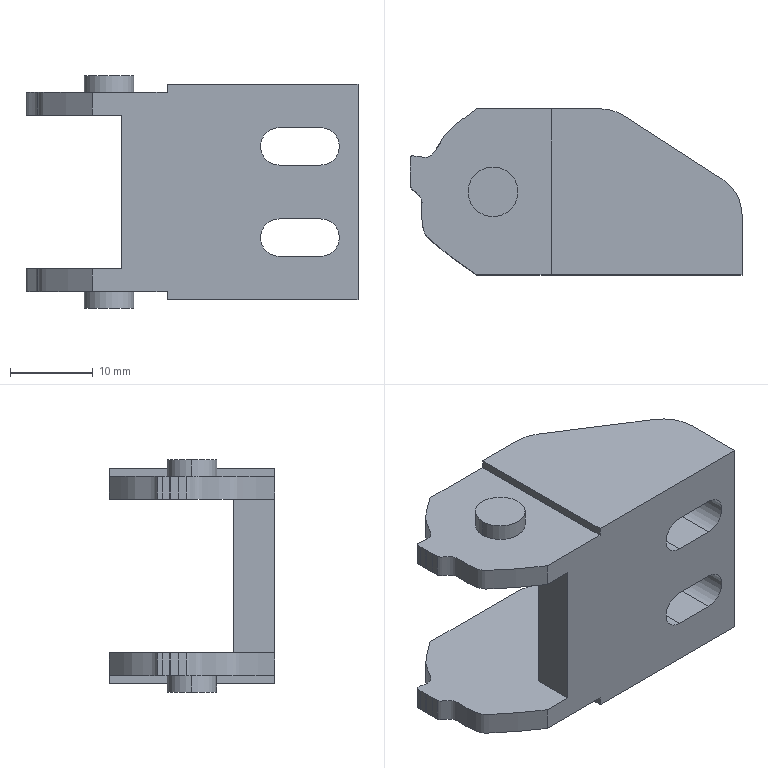Part | STEP file | 1 solid | 48 faces | box 40 x 20 x 28 mm | volume 6776 mm3 | plane 28 | cylinder 12 | spline 8 | commonest cylinder face diameters 4.5 x4 6 x4 10 x4